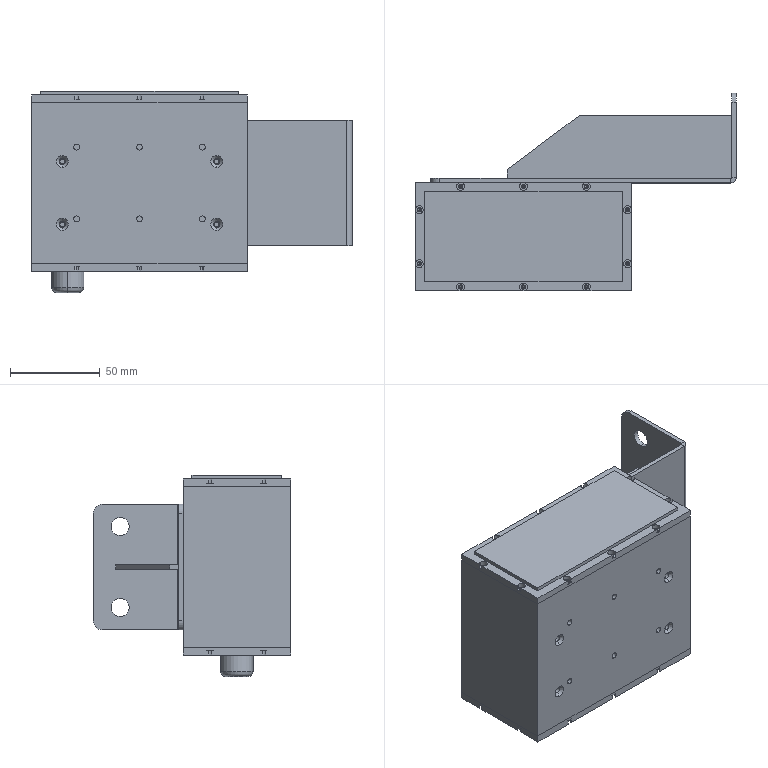Part | SolidWorks | 14 solids | 373 faces | box 178.5 x 110 x 112 mm | volume 250570 mm3 | cylinder 208 | plane 113 | cone 48 | torus 4 | commonest cylinder face diameters 4.4 x42 1.6 x40 2.4 x40 3.3 x24 2.5 x16 3.4 x8